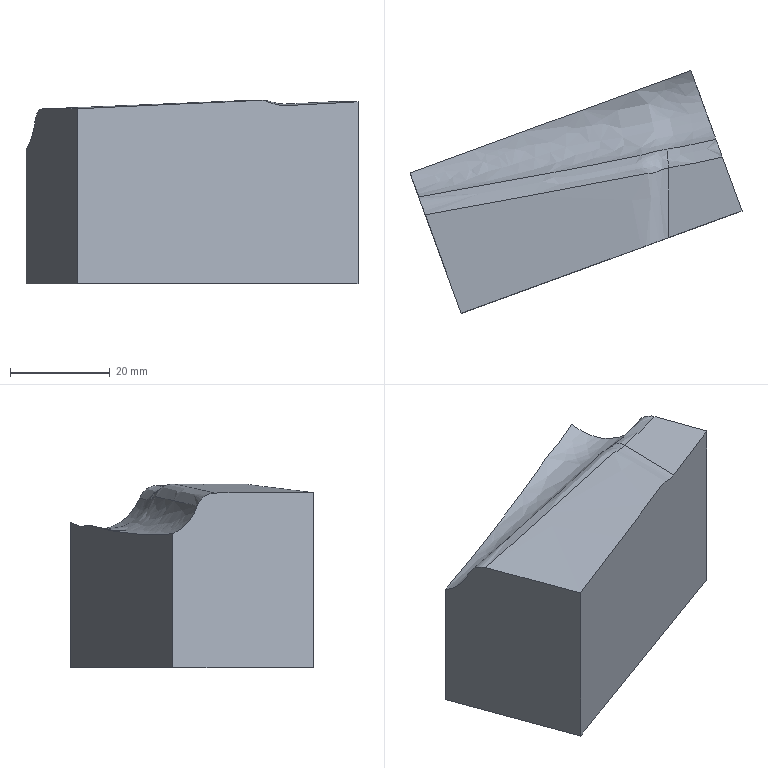Part | NX | features solid 2 | 1 solid | 10 faces | box 66.642 x 48.712 x 36.953 mm | volume 60394 mm3 | plane 5 | spline 5